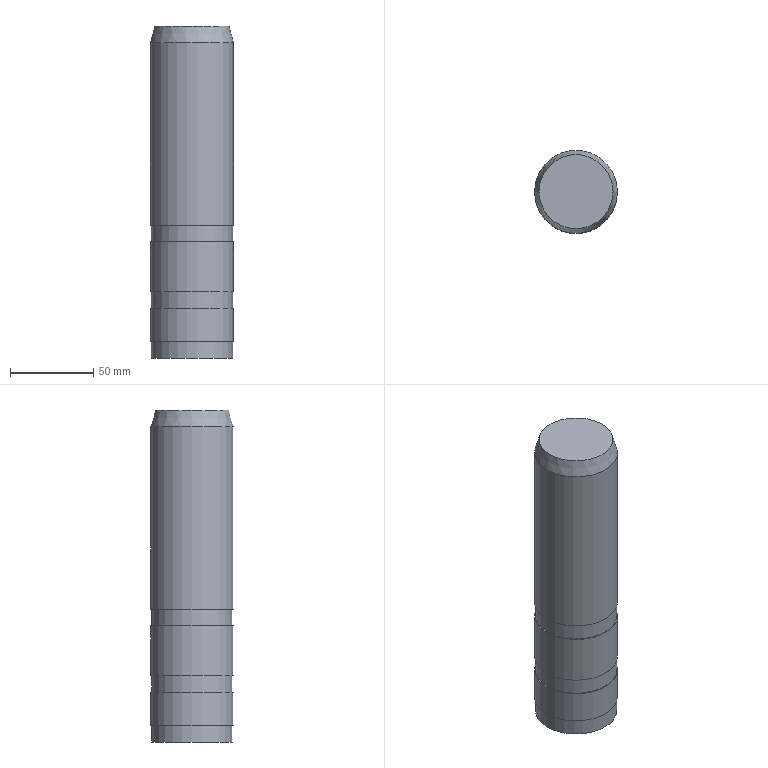Part | NX | features solid 2 | 1 solid | 14 faces | box 50 x 50 x 200 mm | volume 388337 mm3 | plane 7 | cylinder 6 | cone 1 | commonest cylinder face diameters 49 x3 50 x3
STEP:
#1=CARTESIAN_POINT('',(395.5,-220.,-260.));
#2=VERTEX_POINT('',#1);
#3=CARTESIAN_POINT('',(420.,-220.,-260.));
#4=DIRECTION('',(0.,0.,1.));
#5=DIRECTION('',(-1.,0.,0.));
#6=AXIS2_PLACEMENT_3D('',#3,#4,#5);
#7=CIRCLE('',#6,24.5);
#8=EDGE_CURVE('',#2,#2,#7,.T.);
#9=ORIENTED_EDGE('',*,*,#8,.F.);
#10=EDGE_LOOP('',(#9));
#11=FACE_BOUND('',#10,.T.);
#12=CARTESIAN_POINT('',(395.5,-220.,-270.));
#13=VERTEX_POINT('',#12);
#14=CARTESIAN_POINT('',(420.,-220.,-270.));
#15=DIRECTION('',(0.,0.,1.));
#16=DIRECTION('',(-1.,0.,0.));
#17=AXIS2_PLACEMENT_3D('',#14,#15,#16);
#18=CIRCLE('',#17,24.5);
#19=EDGE_CURVE('',#13,#13,#18,.T.);
#20=ORIENTED_EDGE('',*,*,#19,.T.);
#21=EDGE_LOOP('',(#20));
#22=FACE_BOUND('',#21,.T.);
#23=CARTESIAN_POINT('',(420.,-220.,-260.));
#24=DIRECTION('',(0.,0.,-1.));
#25=DIRECTION('',(1.,0.,0.));
#26=AXIS2_PLACEMENT_3D('',#23,#24,#25);
#27=CYLINDRICAL_SURFACE('',#26,24.5);
#28=ADVANCED_FACE('',(#11,#22),#27,.T.);
#29=CARTESIAN_POINT('',(395.,-220.,-260.));
#30=VERTEX_POINT('',#29);
#31=CARTESIAN_POINT('',(420.,-220.,-260.));
#32=DIRECTION('',(0.,0.,1.));
#33=DIRECTION('',(-1.,0.,0.));
#34=AXIS2_PLACEMENT_3D('',#31,#32,#33);
#35=CIRCLE('',#34,25.);
#36=EDGE_CURVE('',#30,#30,#35,.T.);
#37=ORIENTED_EDGE('',*,*,#36,.F.);
#38=EDGE_LOOP('',(#37));
#39=FACE_BOUND('',#38,.T.);
#40=ORIENTED_EDGE('',*,*,#8,.T.);
#41=EDGE_LOOP('',(#40));
#42=FACE_BOUND('',#41,.T.);
#43=CARTESIAN_POINT('',(420.,-220.,-260.));
#44=DIRECTION('',(0.,0.,1.));
#45=DIRECTION('',(-1.,0.,0.));
#46=AXIS2_PLACEMENT_3D('',#43,#44,#45);
#47=PLANE('',#46);
#48=ADVANCED_FACE('',(#39,#42),#47,.F.);
#49=CARTESIAN_POINT('',(395.,-220.,-150.));
#50=VERTEX_POINT('',#49);
#51=CARTESIAN_POINT('',(420.,-220.,-150.));
#52=DIRECTION('',(0.,0.,1.));
#53=DIRECTION('',(-1.,0.,0.));
#54=AXIS2_PLACEMENT_3D('',#51,#52,#53);
#55=CIRCLE('',#54,25.);
#56=EDGE_CURVE('',#50,#50,#55,.T.);
#57=ORIENTED_EDGE('',*,*,#56,.F.);
#58=EDGE_LOOP('',(#57));
#59=FACE_BOUND('',#58,.T.);
#60=ORIENTED_EDGE('',*,*,#36,.T.);
#61=EDGE_LOOP('',(#60));
#62=FACE_BOUND('',#61,.T.);
#63=CARTESIAN_POINT('',(420.,-220.,-190.));
#64=DIRECTION('',(0.,0.,-1.));
#65=DIRECTION('',(1.,0.,0.));
#66=AXIS2_PLACEMENT_3D('',#63,#64,#65);
#67=CYLINDRICAL_SURFACE('',#66,25.);
#68=ADVANCED_FACE('',(#59,#62),#67,.T.);
#69=CARTESIAN_POINT('',(397.679,-220.,-140.));
#70=VERTEX_POINT('',#69);
#71=CARTESIAN_POINT('',(420.,-220.,-140.));
#72=DIRECTION('',(0.,0.,1.));
#73=DIRECTION('',(-1.,0.,0.));
#74=AXIS2_PLACEMENT_3D('',#71,#72,#73);
#75=CIRCLE('',#74,22.321);
#76=EDGE_CURVE('',#70,#70,#75,.T.);
#77=ORIENTED_EDGE('',*,*,#76,.F.);
#78=EDGE_LOOP('',(#77));
#79=FACE_BOUND('',#78,.T.);
#80=ORIENTED_EDGE('',*,*,#56,.T.);
#81=EDGE_LOOP('',(#80));
#82=FACE_BOUND('',#81,.T.);
#83=CARTESIAN_POINT('',(420.,-220.,-150.));
#84=DIRECTION('',(0.,0.,-1.));
#85=DIRECTION('',(-1.,0.,0.));
#86=AXIS2_PLACEMENT_3D('',#83,#84,#85);
#87=CONICAL_SURFACE('',#86,25.,0.2618);
#88=ADVANCED_FACE('',(#79,#82),#87,.T.);
#89=ORIENTED_EDGE('',*,*,#76,.T.);
#90=EDGE_LOOP('',(#89));
#91=FACE_BOUND('',#90,.T.);
#92=CARTESIAN_POINT('',(420.,-220.,-140.));
#93=DIRECTION('',(0.,0.,1.));
#94=DIRECTION('',(-1.,0.,0.));
#95=AXIS2_PLACEMENT_3D('',#92,#93,#94);
#96=PLANE('',#95);
#97=ADVANCED_FACE('',(#91),#96,.T.);
#98=CARTESIAN_POINT('',(395.,-220.,-270.));
#99=VERTEX_POINT('',#98);
#100=CARTESIAN_POINT('',(420.,-220.,-270.));
#101=DIRECTION('',(0.,0.,1.));
#102=DIRECTION('',(-1.,0.,0.));
#103=AXIS2_PLACEMENT_3D('',#100,#101,#102);
#104=CIRCLE('',#103,25.);
#105=EDGE_CURVE('',#99,#99,#104,.T.);
#106=ORIENTED_EDGE('',*,*,#105,.T.);
#107=EDGE_LOOP('',(#106));
#108=FACE_BOUND('',#107,.T.);
#109=ORIENTED_EDGE('',*,*,#19,.F.);
#110=EDGE_LOOP('',(#109));
#111=FACE_BOUND('',#110,.T.);
#112=CARTESIAN_POINT('',(420.,-220.,-270.));
#113=DIRECTION('',(0.,0.,1.));
#114=DIRECTION('',(-1.,0.,0.));
#115=AXIS2_PLACEMENT_3D('',#112,#113,#114);
#116=PLANE('',#115);
#117=ADVANCED_FACE('',(#108,#111),#116,.T.);
#118=CARTESIAN_POINT('',(395.,-220.,-300.));
#119=VERTEX_POINT('',#118);
#120=CARTESIAN_POINT('',(420.,-220.,-300.));
#121=DIRECTION('',(0.,0.,1.));
#122=DIRECTION('',(-1.,0.,0.));
#123=AXIS2_PLACEMENT_3D('',#120,#121,#122);
#124=CIRCLE('',#123,25.);
#125=EDGE_CURVE('',#119,#119,#124,.T.);
#126=ORIENTED_EDGE('',*,*,#125,.T.);
#127=EDGE_LOOP('',(#126));
#128=FACE_BOUND('',#127,.T.);
#129=ORIENTED_EDGE('',*,*,#105,.F.);
#130=EDGE_LOOP('',(#129));
#131=FACE_BOUND('',#130,.T.);
#132=CARTESIAN_POINT('',(420.,-220.,-300.));
#133=DIRECTION('',(0.,0.,1.));
#134=DIRECTION('',(-1.,0.,0.));
#135=AXIS2_PLACEMENT_3D('',#132,#133,#134);
#136=CYLINDRICAL_SURFACE('',#135,25.);
#137=ADVANCED_FACE('',(#128,#131),#136,.T.);
#138=CARTESIAN_POINT('',(395.5,-220.,-300.));
#139=VERTEX_POINT('',#138);
#140=CARTESIAN_POINT('',(420.,-220.,-300.));
#141=DIRECTION('',(0.,0.,1.));
#142=DIRECTION('',(-1.,0.,0.));
#143=AXIS2_PLACEMENT_3D('',#140,#141,#142);
#144=CIRCLE('',#143,24.5);
#145=EDGE_CURVE('',#139,#139,#144,.T.);
#146=ORIENTED_EDGE('',*,*,#145,.T.);
#147=EDGE_LOOP('',(#146));
#148=FACE_BOUND('',#147,.T.);
#149=ORIENTED_EDGE('',*,*,#125,.F.);
#150=EDGE_LOOP('',(#149));
#151=FACE_BOUND('',#150,.T.);
#152=CARTESIAN_POINT('',(420.,-220.,-300.));
#153=DIRECTION('',(0.,0.,1.));
#154=DIRECTION('',(-1.,0.,0.));
#155=AXIS2_PLACEMENT_3D('',#152,#153,#154);
#156=PLANE('',#155);
#157=ADVANCED_FACE('',(#148,#151),#156,.F.);
#158=CARTESIAN_POINT('',(395.5,-220.,-310.));
#159=VERTEX_POINT('',#158);
#160=CARTESIAN_POINT('',(420.,-220.,-310.));
#161=DIRECTION('',(0.,0.,1.));
#162=DIRECTION('',(-1.,0.,0.));
#163=AXIS2_PLACEMENT_3D('',#160,#161,#162);
#164=CIRCLE('',#163,24.5);
#165=EDGE_CURVE('',#159,#159,#164,.F.);
#166=ORIENTED_EDGE('',*,*,#165,.F.);
#167=EDGE_LOOP('',(#166));
#168=FACE_BOUND('',#167,.T.);
#169=ORIENTED_EDGE('',*,*,#145,.F.);
#170=EDGE_LOOP('',(#169));
#171=FACE_BOUND('',#170,.T.);
#172=CARTESIAN_POINT('',(420.,-220.,-310.));
#173=DIRECTION('',(0.,0.,1.));
#174=DIRECTION('',(-1.,0.,0.));
#175=AXIS2_PLACEMENT_3D('',#172,#173,#174);
#176=CYLINDRICAL_SURFACE('',#175,24.5);
#177=ADVANCED_FACE('',(#168,#171),#176,.T.);
#178=CARTESIAN_POINT('',(395.,-220.,-330.));
#179=VERTEX_POINT('',#178);
#180=CARTESIAN_POINT('',(420.,-220.,-330.));
#181=DIRECTION('',(0.,0.,1.));
#182=DIRECTION('',(-1.,0.,0.));
#183=AXIS2_PLACEMENT_3D('',#180,#181,#182);
#184=CIRCLE('',#183,25.);
#185=EDGE_CURVE('',#179,#179,#184,.T.);
#186=ORIENTED_EDGE('',*,*,#185,.T.);
#187=EDGE_LOOP('',(#186));
#188=FACE_BOUND('',#187,.T.);
#189=CARTESIAN_POINT('',(395.,-220.,-310.));
#190=VERTEX_POINT('',#189);
#191=CARTESIAN_POINT('',(420.,-220.,-310.));
#192=DIRECTION('',(0.,0.,1.));
#193=DIRECTION('',(-1.,0.,0.));
#194=AXIS2_PLACEMENT_3D('',#191,#192,#193);
#195=CIRCLE('',#194,25.);
#196=EDGE_CURVE('',#190,#190,#195,.T.);
#197=ORIENTED_EDGE('',*,*,#196,.F.);
#198=EDGE_LOOP('',(#197));
#199=FACE_BOUND('',#198,.T.);
#200=CARTESIAN_POINT('',(420.,-220.,-330.));
#201=DIRECTION('',(0.,0.,1.));
#202=DIRECTION('',(-1.,0.,0.));
#203=AXIS2_PLACEMENT_3D('',#200,#201,#202);
#204=CYLINDRICAL_SURFACE('',#203,25.);
#205=ADVANCED_FACE('',(#188,#199),#204,.T.);
#206=CARTESIAN_POINT('',(395.5,-220.,-330.));
#207=VERTEX_POINT('',#206);
#208=CARTESIAN_POINT('',(420.,-220.,-330.));
#209=DIRECTION('',(0.,0.,1.));
#210=DIRECTION('',(-1.,0.,0.));
#211=AXIS2_PLACEMENT_3D('',#208,#209,#210);
#212=CIRCLE('',#211,24.5);
#213=EDGE_CURVE('',#207,#207,#212,.T.);
#214=ORIENTED_EDGE('',*,*,#213,.T.);
#215=EDGE_LOOP('',(#214));
#216=FACE_BOUND('',#215,.T.);
#217=ORIENTED_EDGE('',*,*,#185,.F.);
#218=EDGE_LOOP('',(#217));
#219=FACE_BOUND('',#218,.T.);
#220=CARTESIAN_POINT('',(420.,-220.,-330.));
#221=DIRECTION('',(0.,0.,1.));
#222=DIRECTION('',(-1.,0.,0.));
#223=AXIS2_PLACEMENT_3D('',#220,#221,#222);
#224=PLANE('',#223);
#225=ADVANCED_FACE('',(#216,#219),#224,.F.);
#226=ORIENTED_EDGE('',*,*,#165,.T.);
#227=EDGE_LOOP('',(#226));
#228=FACE_BOUND('',#227,.T.);
#229=ORIENTED_EDGE('',*,*,#196,.T.);
#230=EDGE_LOOP('',(#229));
#231=FACE_BOUND('',#230,.T.);
#232=CARTESIAN_POINT('',(420.,-220.,-310.));
#233=DIRECTION('',(0.,0.,1.));
#234=DIRECTION('',(-1.,0.,0.));
#235=AXIS2_PLACEMENT_3D('',#232,#233,#234);
#236=PLANE('',#235);
#237=ADVANCED_FACE('',(#228,#231),#236,.T.);
#238=CARTESIAN_POINT('',(395.5,-220.,-340.));
#239=VERTEX_POINT('',#238);
#240=CARTESIAN_POINT('',(420.,-220.,-340.));
#241=DIRECTION('',(0.,0.,1.));
#242=DIRECTION('',(-1.,0.,0.));
#243=AXIS2_PLACEMENT_3D('',#240,#241,#242);
#244=CIRCLE('',#243,24.5);
#245=EDGE_CURVE('',#239,#239,#244,.T.);
#246=ORIENTED_EDGE('',*,*,#245,.T.);
#247=EDGE_LOOP('',(#246));
#248=FACE_BOUND('',#247,.T.);
#249=ORIENTED_EDGE('',*,*,#213,.F.);
#250=EDGE_LOOP('',(#249));
#251=FACE_BOUND('',#250,.T.);
#252=CARTESIAN_POINT('',(420.,-220.,-340.));
#253=DIRECTION('',(0.,0.,1.));
#254=DIRECTION('',(-1.,0.,0.));
#255=AXIS2_PLACEMENT_3D('',#252,#253,#254);
#256=CYLINDRICAL_SURFACE('',#255,24.5);
#257=ADVANCED_FACE('',(#248,#251),#256,.T.);
#258=ORIENTED_EDGE('',*,*,#245,.F.);
#259=EDGE_LOOP('',(#258));
#260=FACE_BOUND('',#259,.T.);
#261=CARTESIAN_POINT('',(420.,-220.,-340.));
#262=DIRECTION('',(0.,0.,1.));
#263=DIRECTION('',(-1.,0.,0.));
#264=AXIS2_PLACEMENT_3D('',#261,#262,#263);
#265=PLANE('',#264);
#266=ADVANCED_FACE('',(#260),#265,.F.);
#267=CLOSED_SHELL('',(#28,#48,#68,#88,#97,#117,#137,#157,#177,#205,#225,#237,#257,#266));
#268=MANIFOLD_SOLID_BREP('',#267);
#269=(LENGTH_UNIT()NAMED_UNIT(*)SI_UNIT(.MILLI.,.METRE.));
#270=UNCERTAINTY_MEASURE_WITH_UNIT(LENGTH_MEASURE(0.00001),#269,'','');
#271=(NAMED_UNIT(*)PLANE_ANGLE_UNIT()SI_UNIT($,.RADIAN.));
#272=(NAMED_UNIT(*)SI_UNIT($,.STERADIAN.)SOLID_ANGLE_UNIT());
#273=(GEOMETRIC_REPRESENTATION_CONTEXT(3)GLOBAL_UNCERTAINTY_ASSIGNED_CONTEXT((#270))GLOBAL_UNIT_ASSIGNED_CONTEXT((#269,#271,#272))REPRESENTATION_CONTEXT('',''));
#274=ADVANCED_BREP_SHAPE_REPRESENTATION('',(#268),#273);